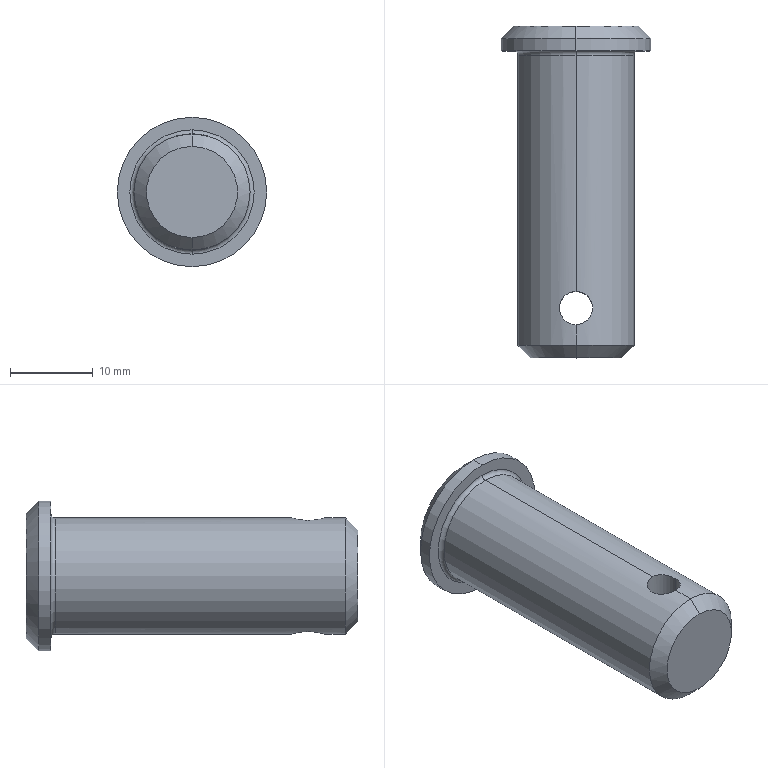Part | SolidWorks | features MirrorStock 1 | 1 solid | 15 faces | box 18 x 40 x 18 mm | volume 6181 mm3 | cylinder 6 | cone 4 | plane 3 | torus 2 | commonest cylinder face diameters 4 x2 14 x2 18 x2
STEP:
#1=CARTESIAN_POINT('',(0.,0.,-7.5));
#2=VERTEX_POINT('',#1);
#3=CARTESIAN_POINT('',(0.,0.,7.5));
#4=VERTEX_POINT('',#3);
#5=CARTESIAN_POINT('',(0.,0.,0.));
#6=DIRECTION('',(0.,-1.,0.));
#7=DIRECTION('',(0.,0.,-1.));
#8=AXIS2_PLACEMENT_3D('',#5,#6,#7);
#9=CIRCLE('',#8,7.5);
#10=EDGE_CURVE('',#2,#4,#9,.T.);
#11=ORIENTED_EDGE('',*,*,#10,.T.);
#12=CARTESIAN_POINT('',(0.,-0.5,7.));
#13=VERTEX_POINT('',#12);
#14=CARTESIAN_POINT('',(0.,-0.5,7.5));
#15=DIRECTION('',(-1.,0.,0.));
#16=DIRECTION('',(0.,0.,1.));
#17=AXIS2_PLACEMENT_3D('',#14,#15,#16);
#18=CIRCLE('',#17,0.5);
#19=EDGE_CURVE('',#4,#13,#18,.T.);
#20=ORIENTED_EDGE('',*,*,#19,.T.);
#21=CARTESIAN_POINT('',(0.,-0.5,-7.));
#22=VERTEX_POINT('',#21);
#23=CARTESIAN_POINT('',(0.,-0.5,0.));
#24=DIRECTION('',(0.,1.,0.));
#25=DIRECTION('',(0.,0.,-1.));
#26=AXIS2_PLACEMENT_3D('',#23,#24,#25);
#27=CIRCLE('',#26,7.);
#28=EDGE_CURVE('',#13,#22,#27,.T.);
#29=ORIENTED_EDGE('',*,*,#28,.T.);
#30=CARTESIAN_POINT('',(0.,-0.5,-7.5));
#31=DIRECTION('',(1.,0.,0.));
#32=DIRECTION('',(0.,0.,-1.));
#33=AXIS2_PLACEMENT_3D('',#30,#31,#32);
#34=CIRCLE('',#33,0.5);
#35=EDGE_CURVE('',#2,#22,#34,.T.);
#36=ORIENTED_EDGE('',*,*,#35,.F.);
#37=EDGE_LOOP('',(#11,#20,#29,#36));
#38=FACE_OUTER_BOUND('',#37,.T.);
#39=CARTESIAN_POINT('',(0.,-0.5,0.));
#40=DIRECTION('',(0.,1.,0.));
#41=DIRECTION('',(0.,0.,-1.));
#42=AXIS2_PLACEMENT_3D('',#39,#40,#41);
#43=TOROIDAL_SURFACE('',#42,7.5,0.5);
#44=ADVANCED_FACE('',(#38),#43,.F.);
#45=CARTESIAN_POINT('',(0.,-29.,7.));
#46=VERTEX_POINT('',#45);
#47=CARTESIAN_POINT('',(-2.,-31.,6.708));
#48=VERTEX_POINT('',#47);
#49=CARTESIAN_POINT('',(0.,-29.,7.));
#50=CARTESIAN_POINT('',(-0.1312,-29.,7.));
#51=CARTESIAN_POINT('',(-0.2645,-29.013,6.996));
#52=CARTESIAN_POINT('',(-0.5215,-29.065,6.982));
#53=CARTESIAN_POINT('',(-0.6465,-29.103,6.971));
#54=CARTESIAN_POINT('',(-1.011,-29.254,6.931));
#55=CARTESIAN_POINT('',(-1.231,-29.402,6.894));
#56=CARTESIAN_POINT('',(-1.507,-29.679,6.836));
#57=CARTESIAN_POINT('',(-1.59,-29.779,6.818));
#58=CARTESIAN_POINT('',(-1.734,-29.995,6.782));
#59=CARTESIAN_POINT('',(-1.797,-30.113,6.766));
#60=CARTESIAN_POINT('',(-1.897,-30.354,6.738));
#61=CARTESIAN_POINT('',(-1.935,-30.478,6.727));
#62=CARTESIAN_POINT('',(-1.987,-30.736,6.712));
#63=CARTESIAN_POINT('',(-2.,-30.869,6.708));
#64=CARTESIAN_POINT('',(-2.,-31.,6.708));
#65=B_SPLINE_CURVE_WITH_KNOTS('',3,(#49,#50,#51,#52,#53,#54,#55,#56,#57,#58,#59,#60,#61,#62,#63,#64),.UNSPECIFIED.,.F.,.F.,(4,2,2,2,2,2,2,4),(0.003144,0.003536,0.003929,0.004715,0.005107,0.0055,0.005893,0.006286),.UNSPECIFIED.);
#66=EDGE_CURVE('',#46,#48,#65,.T.);
#67=ORIENTED_EDGE('',*,*,#66,.T.);
#68=CARTESIAN_POINT('',(-2.,-31.,-6.708));
#69=VERTEX_POINT('',#68);
#70=CARTESIAN_POINT('',(-2.,-31.,9.));
#71=DIRECTION('',(0.,0.,-1.));
#72=VECTOR('',#71,1000.);
#73=LINE('',#70,#72);
#74=EDGE_CURVE('',#48,#69,#73,.T.);
#75=ORIENTED_EDGE('',*,*,#74,.T.);
#76=CARTESIAN_POINT('',(0.,-29.,-7.));
#77=VERTEX_POINT('',#76);
#78=CARTESIAN_POINT('',(-2.,-31.,-6.708));
#79=CARTESIAN_POINT('',(-2.,-30.869,-6.708));
#80=CARTESIAN_POINT('',(-1.987,-30.736,-6.712));
#81=CARTESIAN_POINT('',(-1.935,-30.479,-6.727));
#82=CARTESIAN_POINT('',(-1.897,-30.354,-6.738));
#83=CARTESIAN_POINT('',(-1.746,-29.989,-6.78));
#84=CARTESIAN_POINT('',(-1.598,-29.77,-6.818));
#85=CARTESIAN_POINT('',(-1.321,-29.493,-6.875));
#86=CARTESIAN_POINT('',(-1.221,-29.41,-6.894));
#87=CARTESIAN_POINT('',(-1.005,-29.266,-6.928));
#88=CARTESIAN_POINT('',(-0.8876,-29.203,-6.945));
#89=CARTESIAN_POINT('',(-0.6464,-29.103,-6.971));
#90=CARTESIAN_POINT('',(-0.5217,-29.065,-6.982));
#91=CARTESIAN_POINT('',(-0.2636,-29.013,-6.996));
#92=CARTESIAN_POINT('',(-0.1309,-29.,-7.));
#93=CARTESIAN_POINT('',(0.,-29.,-7.));
#94=B_SPLINE_CURVE_WITH_KNOTS('',3,(#78,#79,#80,#81,#82,#83,#84,#85,#86,#87,#88,#89,#90,#91,#92,#93),.UNSPECIFIED.,.F.,.F.,(4,2,2,2,2,2,2,4),(0.003144,0.003537,0.003929,0.004715,0.005108,0.0055,0.005893,0.006286),.UNSPECIFIED.);
#95=EDGE_CURVE('',#69,#77,#94,.T.);
#96=ORIENTED_EDGE('',*,*,#95,.T.);
#97=CARTESIAN_POINT('',(2.,-31.,-6.708));
#98=VERTEX_POINT('',#97);
#99=CARTESIAN_POINT('',(0.,-29.,-7.));
#100=CARTESIAN_POINT('',(0.2619,-29.,-7.));
#101=CARTESIAN_POINT('',(0.5263,-29.053,-6.984));
#102=CARTESIAN_POINT('',(0.8879,-29.203,-6.945));
#103=CARTESIAN_POINT('',(1.005,-29.266,-6.928));
#104=CARTESIAN_POINT('',(1.222,-29.411,-6.893));
#105=CARTESIAN_POINT('',(1.322,-29.493,-6.875));
#106=CARTESIAN_POINT('',(1.506,-29.678,-6.837));
#107=CARTESIAN_POINT('',(1.59,-29.78,-6.817));
#108=CARTESIAN_POINT('',(1.734,-29.995,-6.782));
#109=CARTESIAN_POINT('',(1.796,-30.11,-6.766));
#110=CARTESIAN_POINT('',(1.897,-30.354,-6.738));
#111=CARTESIAN_POINT('',(1.935,-30.479,-6.727));
#112=CARTESIAN_POINT('',(1.987,-30.735,-6.712));
#113=CARTESIAN_POINT('',(2.,-30.868,-6.708));
#114=CARTESIAN_POINT('',(2.,-31.,-6.708));
#115=B_SPLINE_CURVE_WITH_KNOTS('',3,(#99,#100,#101,#102,#103,#104,#105,#106,#107,#108,#109,#110,#111,#112,#113,#114),.UNSPECIFIED.,.F.,.F.,(4,2,2,2,2,2,2,4),(0.006286,0.007071,0.007464,0.007857,0.00825,0.008643,0.009035,0.009428),.UNSPECIFIED.);
#116=EDGE_CURVE('',#77,#98,#115,.T.);
#117=ORIENTED_EDGE('',*,*,#116,.T.);
#118=CARTESIAN_POINT('',(2.,-31.,6.708));
#119=VERTEX_POINT('',#118);
#120=CARTESIAN_POINT('',(2.,-31.,9.));
#121=DIRECTION('',(0.,0.,-1.));
#122=VECTOR('',#121,1000.);
#123=LINE('',#120,#122);
#124=EDGE_CURVE('',#119,#98,#123,.T.);
#125=ORIENTED_EDGE('',*,*,#124,.F.);
#126=CARTESIAN_POINT('',(2.,-31.,6.708));
#127=CARTESIAN_POINT('',(2.,-30.867,6.708));
#128=CARTESIAN_POINT('',(1.987,-30.737,6.712));
#129=CARTESIAN_POINT('',(1.936,-30.48,6.727));
#130=CARTESIAN_POINT('',(1.897,-30.352,6.738));
#131=CARTESIAN_POINT('',(1.796,-30.111,6.766));
#132=CARTESIAN_POINT('',(1.735,-29.996,6.782));
#133=CARTESIAN_POINT('',(1.589,-29.779,6.818));
#134=CARTESIAN_POINT('',(1.505,-29.677,6.837));
#135=CARTESIAN_POINT('',(1.23,-29.402,6.894));
#136=CARTESIAN_POINT('',(1.008,-29.253,6.931));
#137=CARTESIAN_POINT('',(0.6471,-29.103,6.971));
#138=CARTESIAN_POINT('',(0.5202,-29.064,6.982));
#139=CARTESIAN_POINT('',(0.2616,-29.013,6.996));
#140=CARTESIAN_POINT('',(0.1313,-29.,7.));
#141=CARTESIAN_POINT('',(0.,-29.,7.));
#142=B_SPLINE_CURVE_WITH_KNOTS('',3,(#126,#127,#128,#129,#130,#131,#132,#133,#134,#135,#136,#137,#138,#139,#140,#141),.UNSPECIFIED.,.F.,.F.,(4,2,2,2,2,2,2,4),(0.,0.000393,0.0007859,0.001179,0.001572,0.002358,0.002751,0.003144),.UNSPECIFIED.);
#143=EDGE_CURVE('',#119,#46,#142,.T.);
#144=ORIENTED_EDGE('',*,*,#143,.T.);
#145=EDGE_LOOP('',(#67,#75,#96,#117,#125,#144));
#146=FACE_OUTER_BOUND('',#145,.T.);
#147=CARTESIAN_POINT('',(0.,-31.,9.));
#148=DIRECTION('',(0.,0.,-1.));
#149=DIRECTION('',(1.,0.,0.));
#150=AXIS2_PLACEMENT_3D('',#147,#148,#149);
#151=CYLINDRICAL_SURFACE('',#150,2.);
#152=ADVANCED_FACE('',(#146),#151,.F.);
#153=CARTESIAN_POINT('',(0.,3.,7.5));
#154=VERTEX_POINT('',#153);
#155=CARTESIAN_POINT('',(0.,3.,-7.5));
#156=VERTEX_POINT('',#155);
#157=CARTESIAN_POINT('',(0.,3.,0.));
#158=DIRECTION('',(0.,-1.,0.));
#159=DIRECTION('',(0.,0.,-1.));
#160=AXIS2_PLACEMENT_3D('',#157,#158,#159);
#161=CIRCLE('',#160,7.5);
#162=EDGE_CURVE('',#154,#156,#161,.T.);
#163=ORIENTED_EDGE('',*,*,#162,.T.);
#164=CARTESIAN_POINT('',(0.,1.5,-9.));
#165=VERTEX_POINT('',#164);
#166=CARTESIAN_POINT('',(0.,3.,-7.5));
#167=DIRECTION('',(0.,-0.7071,-0.7071));
#168=VECTOR('',#167,1000.);
#169=LINE('',#166,#168);
#170=EDGE_CURVE('',#156,#165,#169,.T.);
#171=ORIENTED_EDGE('',*,*,#170,.T.);
#172=CARTESIAN_POINT('',(0.,1.5,9.));
#173=VERTEX_POINT('',#172);
#174=CARTESIAN_POINT('',(0.,1.5,0.));
#175=DIRECTION('',(0.,1.,0.));
#176=DIRECTION('',(0.,0.,-1.));
#177=AXIS2_PLACEMENT_3D('',#174,#175,#176);
#178=CIRCLE('',#177,9.);
#179=EDGE_CURVE('',#165,#173,#178,.T.);
#180=ORIENTED_EDGE('',*,*,#179,.T.);
#181=CARTESIAN_POINT('',(0.,3.,7.5));
#182=DIRECTION('',(0.,-0.7071,0.7071));
#183=VECTOR('',#182,1000.);
#184=LINE('',#181,#183);
#185=EDGE_CURVE('',#154,#173,#184,.T.);
#186=ORIENTED_EDGE('',*,*,#185,.F.);
#187=EDGE_LOOP('',(#163,#171,#180,#186));
#188=FACE_OUTER_BOUND('',#187,.T.);
#189=CARTESIAN_POINT('',(0.,3.,0.));
#190=DIRECTION('',(0.,-1.,0.));
#191=DIRECTION('',(0.,0.,1.));
#192=AXIS2_PLACEMENT_3D('',#189,#190,#191);
#193=CONICAL_SURFACE('',#192,7.5,0.7854);
#194=ADVANCED_FACE('',(#188),#193,.T.);
#195=CARTESIAN_POINT('',(0.,-37.,-5.5));
#196=VERTEX_POINT('',#195);
#197=CARTESIAN_POINT('',(0.,-37.,5.5));
#198=VERTEX_POINT('',#197);
#199=CARTESIAN_POINT('',(0.,-37.,0.));
#200=DIRECTION('',(0.,1.,0.));
#201=DIRECTION('',(0.,0.,1.));
#202=AXIS2_PLACEMENT_3D('',#199,#200,#201);
#203=CIRCLE('',#202,5.5);
#204=EDGE_CURVE('',#196,#198,#203,.T.);
#205=ORIENTED_EDGE('',*,*,#204,.T.);
#206=CARTESIAN_POINT('',(0.,-35.5,7.));
#207=VERTEX_POINT('',#206);
#208=CARTESIAN_POINT('',(0.,-37.,5.5));
#209=DIRECTION('',(0.,0.7071,0.7071));
#210=VECTOR('',#209,1000.);
#211=LINE('',#208,#210);
#212=EDGE_CURVE('',#198,#207,#211,.T.);
#213=ORIENTED_EDGE('',*,*,#212,.T.);
#214=CARTESIAN_POINT('',(0.,-35.5,-7.));
#215=VERTEX_POINT('',#214);
#216=CARTESIAN_POINT('',(0.,-35.5,0.));
#217=DIRECTION('',(0.,-1.,0.));
#218=DIRECTION('',(0.,0.,1.));
#219=AXIS2_PLACEMENT_3D('',#216,#217,#218);
#220=CIRCLE('',#219,7.);
#221=EDGE_CURVE('',#207,#215,#220,.T.);
#222=ORIENTED_EDGE('',*,*,#221,.T.);
#223=CARTESIAN_POINT('',(0.,-37.,-5.5));
#224=DIRECTION('',(0.,0.7071,-0.7071));
#225=VECTOR('',#224,1000.);
#226=LINE('',#223,#225);
#227=EDGE_CURVE('',#196,#215,#226,.T.);
#228=ORIENTED_EDGE('',*,*,#227,.F.);
#229=EDGE_LOOP('',(#205,#213,#222,#228));
#230=FACE_OUTER_BOUND('',#229,.T.);
#231=CARTESIAN_POINT('',(0.,-37.,0.));
#232=DIRECTION('',(0.,1.,0.));
#233=DIRECTION('',(0.,0.,-1.));
#234=AXIS2_PLACEMENT_3D('',#231,#232,#233);
#235=CONICAL_SURFACE('',#234,5.5,0.7854);
#236=ADVANCED_FACE('',(#230),#235,.T.);
#237=ORIENTED_EDGE('',*,*,#221,.F.);
#238=CARTESIAN_POINT('',(0.,-33.,7.));
#239=VERTEX_POINT('',#238);
#240=CARTESIAN_POINT('',(0.,-37.,7.));
#241=DIRECTION('',(0.,1.,0.));
#242=VECTOR('',#241,1000.);
#243=LINE('',#240,#242);
#244=EDGE_CURVE('',#207,#239,#243,.T.);
#245=ORIENTED_EDGE('',*,*,#244,.T.);
#246=CARTESIAN_POINT('',(-2.,-31.,6.708));
#247=CARTESIAN_POINT('',(-2.,-31.262,6.708));
#248=CARTESIAN_POINT('',(-1.947,-31.526,6.725));
#249=CARTESIAN_POINT('',(-1.797,-31.888,6.766));
#250=CARTESIAN_POINT('',(-1.734,-32.005,6.782));
#251=CARTESIAN_POINT('',(-1.589,-32.221,6.818));
#252=CARTESIAN_POINT('',(-1.507,-32.322,6.837));
#253=CARTESIAN_POINT('',(-1.322,-32.506,6.875));
#254=CARTESIAN_POINT('',(-1.22,-32.59,6.894));
#255=CARTESIAN_POINT('',(-1.005,-32.734,6.928));
#256=CARTESIAN_POINT('',(-0.89,-32.796,6.944));
#257=CARTESIAN_POINT('',(-0.646,-32.897,6.971));
#258=CARTESIAN_POINT('',(-0.5208,-32.935,6.982));
#259=CARTESIAN_POINT('',(-0.2645,-32.987,6.996));
#260=CARTESIAN_POINT('',(-0.1318,-33.,7.));
#261=CARTESIAN_POINT('',(0.,-33.,7.));
#262=B_SPLINE_CURVE_WITH_KNOTS('',3,(#246,#247,#248,#249,#250,#251,#252,#253,#254,#255,#256,#257,#258,#259,#260,#261),.UNSPECIFIED.,.F.,.F.,(4,2,2,2,2,2,2,4),(0.006286,0.007071,0.007464,0.007857,0.00825,0.008642,0.009035,0.009428),.UNSPECIFIED.);
#263=EDGE_CURVE('',#48,#239,#262,.T.);
#264=ORIENTED_EDGE('',*,*,#263,.F.);
#265=ORIENTED_EDGE('',*,*,#66,.F.);
#266=CARTESIAN_POINT('',(0.,-37.,7.));
#267=DIRECTION('',(0.,1.,0.));
#268=VECTOR('',#267,1000.);
#269=LINE('',#266,#268);
#270=EDGE_CURVE('',#46,#13,#269,.T.);
#271=ORIENTED_EDGE('',*,*,#270,.T.);
#272=CARTESIAN_POINT('',(0.,-0.5,0.));
#273=DIRECTION('',(0.,1.,0.));
#274=DIRECTION('',(0.,0.,-1.));
#275=AXIS2_PLACEMENT_3D('',#272,#273,#274);
#276=CIRCLE('',#275,7.);
#277=EDGE_CURVE('',#22,#13,#276,.T.);
#278=ORIENTED_EDGE('',*,*,#277,.F.);
#279=CARTESIAN_POINT('',(0.,-37.,-7.));
#280=DIRECTION('',(0.,1.,0.));
#281=VECTOR('',#280,1000.);
#282=LINE('',#279,#281);
#283=EDGE_CURVE('',#77,#22,#282,.T.);
#284=ORIENTED_EDGE('',*,*,#283,.F.);
#285=ORIENTED_EDGE('',*,*,#95,.F.);
#286=CARTESIAN_POINT('',(0.,-33.,-7.));
#287=VERTEX_POINT('',#286);
#288=CARTESIAN_POINT('',(0.,-33.,-7.));
#289=CARTESIAN_POINT('',(-0.1329,-33.,-7.));
#290=CARTESIAN_POINT('',(-0.2635,-32.987,-6.996));
#291=CARTESIAN_POINT('',(-0.5202,-32.936,-6.982));
#292=CARTESIAN_POINT('',(-0.6476,-32.897,-6.971));
#293=CARTESIAN_POINT('',(-0.8896,-32.796,-6.944));
#294=CARTESIAN_POINT('',(-1.004,-32.735,-6.928));
#295=CARTESIAN_POINT('',(-1.221,-32.589,-6.894));
#296=CARTESIAN_POINT('',(-1.323,-32.505,-6.874));
#297=CARTESIAN_POINT('',(-1.598,-32.23,-6.818));
#298=CARTESIAN_POINT('',(-1.747,-32.008,-6.779));
#299=CARTESIAN_POINT('',(-1.897,-31.647,-6.738));
#300=CARTESIAN_POINT('',(-1.936,-31.52,-6.727));
#301=CARTESIAN_POINT('',(-1.987,-31.262,-6.712));
#302=CARTESIAN_POINT('',(-2.,-31.131,-6.708));
#303=CARTESIAN_POINT('',(-2.,-31.,-6.708));
#304=B_SPLINE_CURVE_WITH_KNOTS('',3,(#288,#289,#290,#291,#292,#293,#294,#295,#296,#297,#298,#299,#300,#301,#302,#303),.UNSPECIFIED.,.F.,.F.,(4,2,2,2,2,2,2,4),(0.,0.000393,0.000786,0.001179,0.001572,0.002358,0.002751,0.003144),.UNSPECIFIED.);
#305=EDGE_CURVE('',#287,#69,#304,.T.);
#306=ORIENTED_EDGE('',*,*,#305,.F.);
#307=CARTESIAN_POINT('',(0.,-37.,-7.));
#308=DIRECTION('',(0.,1.,0.));
#309=VECTOR('',#308,1000.);
#310=LINE('',#307,#309);
#311=EDGE_CURVE('',#215,#287,#310,.T.);
#312=ORIENTED_EDGE('',*,*,#311,.F.);
#313=EDGE_LOOP('',(#237,#245,#264,#265,#271,#278,#284,#285,#306,#312));
#314=FACE_OUTER_BOUND('',#313,.T.);
#315=CARTESIAN_POINT('',(0.,-37.,0.));
#316=DIRECTION('',(0.,1.,0.));
#317=DIRECTION('',(0.,0.,-1.));
#318=AXIS2_PLACEMENT_3D('',#315,#316,#317);
#319=CYLINDRICAL_SURFACE('',#318,7.);
#320=ADVANCED_FACE('',(#314),#319,.T.);
#321=ORIENTED_EDGE('',*,*,#179,.F.);
#322=CARTESIAN_POINT('',(0.,0.,-9.));
#323=VERTEX_POINT('',#322);
#324=CARTESIAN_POINT('',(0.,3.,-9.));
#325=DIRECTION('',(0.,-1.,0.));
#326=VECTOR('',#325,1000.);
#327=LINE('',#324,#326);
#328=EDGE_CURVE('',#165,#323,#327,.T.);
#329=ORIENTED_EDGE('',*,*,#328,.T.);
#330=CARTESIAN_POINT('',(0.,0.,9.));
#331=VERTEX_POINT('',#330);
#332=CARTESIAN_POINT('',(0.,0.,0.));
#333=DIRECTION('',(0.,-1.,0.));
#334=DIRECTION('',(0.,0.,-1.));
#335=AXIS2_PLACEMENT_3D('',#332,#333,#334);
#336=CIRCLE('',#335,9.);
#337=EDGE_CURVE('',#331,#323,#336,.T.);
#338=ORIENTED_EDGE('',*,*,#337,.F.);
#339=CARTESIAN_POINT('',(0.,3.,9.));
#340=DIRECTION('',(0.,-1.,0.));
#341=VECTOR('',#340,1000.);
#342=LINE('',#339,#341);
#343=EDGE_CURVE('',#173,#331,#342,.T.);
#344=ORIENTED_EDGE('',*,*,#343,.F.);
#345=EDGE_LOOP('',(#321,#329,#338,#344));
#346=FACE_OUTER_BOUND('',#345,.T.);
#347=CARTESIAN_POINT('',(0.,3.,0.));
#348=DIRECTION('',(0.,-1.,0.));
#349=DIRECTION('',(0.,0.,1.));
#350=AXIS2_PLACEMENT_3D('',#347,#348,#349);
#351=CYLINDRICAL_SURFACE('',#350,9.);
#352=ADVANCED_FACE('',(#346),#351,.T.);
#353=ORIENTED_EDGE('',*,*,#328,.F.);
#354=CARTESIAN_POINT('',(0.,1.5,0.));
#355=DIRECTION('',(0.,1.,0.));
#356=DIRECTION('',(0.,0.,-1.));
#357=AXIS2_PLACEMENT_3D('',#354,#355,#356);
#358=CIRCLE('',#357,9.);
#359=EDGE_CURVE('',#173,#165,#358,.T.);
#360=ORIENTED_EDGE('',*,*,#359,.F.);
#361=ORIENTED_EDGE('',*,*,#343,.T.);
#362=CARTESIAN_POINT('',(0.,0.,0.));
#363=DIRECTION('',(0.,-1.,0.));
#364=DIRECTION('',(0.,0.,-1.));
#365=AXIS2_PLACEMENT_3D('',#362,#363,#364);
#366=CIRCLE('',#365,9.);
#367=EDGE_CURVE('',#323,#331,#366,.T.);
#368=ORIENTED_EDGE('',*,*,#367,.F.);
#369=EDGE_LOOP('',(#353,#360,#361,#368));
#370=FACE_OUTER_BOUND('',#369,.T.);
#371=CARTESIAN_POINT('',(0.,3.,0.));
#372=DIRECTION('',(0.,-1.,0.));
#373=DIRECTION('',(0.,0.,1.));
#374=AXIS2_PLACEMENT_3D('',#371,#372,#373);
#375=CYLINDRICAL_SURFACE('',#374,9.);
#376=ADVANCED_FACE('',(#370),#375,.T.);
#377=ORIENTED_EDGE('',*,*,#162,.F.);
#378=CARTESIAN_POINT('',(0.,3.,0.));
#379=DIRECTION('',(0.,-1.,0.));
#380=DIRECTION('',(0.,0.,-1.));
#381=AXIS2_PLACEMENT_3D('',#378,#379,#380);
#382=CIRCLE('',#381,7.5);
#383=EDGE_CURVE('',#156,#154,#382,.T.);
#384=ORIENTED_EDGE('',*,*,#383,.F.);
#385=EDGE_LOOP('',(#377,#384));
#386=FACE_OUTER_BOUND('',#385,.T.);
#387=CARTESIAN_POINT('',(0.,3.,0.));
#388=DIRECTION('',(0.,1.,0.));
#389=DIRECTION('',(0.,0.,-1.));
#390=AXIS2_PLACEMENT_3D('',#387,#388,#389);
#391=PLANE('',#390);
#392=ADVANCED_FACE('',(#386),#391,.T.);
#393=ORIENTED_EDGE('',*,*,#10,.F.);
#394=CARTESIAN_POINT('',(0.,0.,0.));
#395=DIRECTION('',(0.,-1.,0.));
#396=DIRECTION('',(0.,0.,-1.));
#397=AXIS2_PLACEMENT_3D('',#394,#395,#396);
#398=CIRCLE('',#397,7.5);
#399=EDGE_CURVE('',#4,#2,#398,.T.);
#400=ORIENTED_EDGE('',*,*,#399,.F.);
#401=EDGE_LOOP('',(#393,#400));
#402=FACE_BOUND('',#401,.T.);
#403=ORIENTED_EDGE('',*,*,#337,.T.);
#404=ORIENTED_EDGE('',*,*,#367,.T.);
#405=EDGE_LOOP('',(#403,#404));
#406=FACE_OUTER_BOUND('',#405,.T.);
#407=CARTESIAN_POINT('',(0.,0.,0.));
#408=DIRECTION('',(0.,1.,0.));
#409=DIRECTION('',(0.,0.,-1.));
#410=AXIS2_PLACEMENT_3D('',#407,#408,#409);
#411=PLANE('',#410);
#412=ADVANCED_FACE('',(#402,#406),#411,.F.);
#413=ORIENTED_EDGE('',*,*,#244,.F.);
#414=CARTESIAN_POINT('',(0.,-35.5,0.));
#415=DIRECTION('',(0.,-1.,0.));
#416=DIRECTION('',(0.,0.,1.));
#417=AXIS2_PLACEMENT_3D('',#414,#415,#416);
#418=CIRCLE('',#417,7.);
#419=EDGE_CURVE('',#215,#207,#418,.T.);
#420=ORIENTED_EDGE('',*,*,#419,.F.);
#421=ORIENTED_EDGE('',*,*,#311,.T.);
#422=CARTESIAN_POINT('',(2.,-31.,-6.708));
#423=CARTESIAN_POINT('',(2.,-31.132,-6.708));
#424=CARTESIAN_POINT('',(1.987,-31.262,-6.712));
#425=CARTESIAN_POINT('',(1.936,-31.519,-6.727));
#426=CARTESIAN_POINT('',(1.897,-31.647,-6.738));
#427=CARTESIAN_POINT('',(1.747,-32.008,-6.779));
#428=CARTESIAN_POINT('',(1.598,-32.23,-6.818));
#429=CARTESIAN_POINT('',(1.323,-32.505,-6.874));
#430=CARTESIAN_POINT('',(1.221,-32.589,-6.894));
#431=CARTESIAN_POINT('',(1.004,-32.735,-6.928));
#432=CARTESIAN_POINT('',(0.8896,-32.796,-6.944));
#433=CARTESIAN_POINT('',(0.6486,-32.896,-6.971));
#434=CARTESIAN_POINT('',(0.521,-32.935,-6.982));
#435=CARTESIAN_POINT('',(0.2636,-32.987,-6.996));
#436=CARTESIAN_POINT('',(0.1328,-33.,-7.));
#437=CARTESIAN_POINT('',(0.,-33.,-7.));
#438=B_SPLINE_CURVE_WITH_KNOTS('',3,(#422,#423,#424,#425,#426,#427,#428,#429,#430,#431,#432,#433,#434,#435,#436,#437),.UNSPECIFIED.,.F.,.F.,(4,2,2,2,2,2,2,4),(0.009428,0.009821,0.01021,0.011,0.01139,0.01178,0.01218,0.01257),.UNSPECIFIED.);
#439=EDGE_CURVE('',#98,#287,#438,.T.);
#440=ORIENTED_EDGE('',*,*,#439,.F.);
#441=ORIENTED_EDGE('',*,*,#116,.F.);
#442=ORIENTED_EDGE('',*,*,#283,.T.);
#443=ORIENTED_EDGE('',*,*,#28,.F.);
#444=ORIENTED_EDGE('',*,*,#270,.F.);
#445=ORIENTED_EDGE('',*,*,#143,.F.);
#446=CARTESIAN_POINT('',(0.,-33.,7.));
#447=CARTESIAN_POINT('',(0.1318,-33.,7.));
#448=CARTESIAN_POINT('',(0.2621,-32.987,6.996));
#449=CARTESIAN_POINT('',(0.5195,-32.936,6.982));
#450=CARTESIAN_POINT('',(0.6471,-32.897,6.971));
#451=CARTESIAN_POINT('',(1.009,-32.747,6.931));
#452=CARTESIAN_POINT('',(1.23,-32.598,6.894));
#453=CARTESIAN_POINT('',(1.506,-32.323,6.837));
#454=CARTESIAN_POINT('',(1.589,-32.221,6.818));
#455=CARTESIAN_POINT('',(1.735,-32.004,6.782));
#456=CARTESIAN_POINT('',(1.796,-31.89,6.766));
#457=CARTESIAN_POINT('',(1.896,-31.649,6.738));
#458=CARTESIAN_POINT('',(1.935,-31.521,6.727));
#459=CARTESIAN_POINT('',(1.987,-31.264,6.712));
#460=CARTESIAN_POINT('',(2.,-31.133,6.708));
#461=CARTESIAN_POINT('',(2.,-31.,6.708));
#462=B_SPLINE_CURVE_WITH_KNOTS('',3,(#446,#447,#448,#449,#450,#451,#452,#453,#454,#455,#456,#457,#458,#459,#460,#461),.UNSPECIFIED.,.F.,.F.,(4,2,2,2,2,2,2,4),(0.009428,0.009821,0.01021,0.011,0.01139,0.01178,0.01218,0.01257),.UNSPECIFIED.);
#463=EDGE_CURVE('',#239,#119,#462,.T.);
#464=ORIENTED_EDGE('',*,*,#463,.F.);
#465=EDGE_LOOP('',(#413,#420,#421,#440,#441,#442,#443,#444,#445,#464));
#466=FACE_OUTER_BOUND('',#465,.T.);
#467=CARTESIAN_POINT('',(0.,-37.,0.));
#468=DIRECTION('',(0.,1.,0.));
#469=DIRECTION('',(0.,0.,-1.));
#470=AXIS2_PLACEMENT_3D('',#467,#468,#469);
#471=CYLINDRICAL_SURFACE('',#470,7.);
#472=ADVANCED_FACE('',(#466),#471,.T.);
#473=ORIENTED_EDGE('',*,*,#204,.F.);
#474=CARTESIAN_POINT('',(0.,-37.,0.));
#475=DIRECTION('',(0.,1.,0.));
#476=DIRECTION('',(0.,0.,1.));
#477=AXIS2_PLACEMENT_3D('',#474,#475,#476);
#478=CIRCLE('',#477,5.5);
#479=EDGE_CURVE('',#198,#196,#478,.T.);
#480=ORIENTED_EDGE('',*,*,#479,.F.);
#481=EDGE_LOOP('',(#473,#480));
#482=FACE_OUTER_BOUND('',#481,.T.);
#483=CARTESIAN_POINT('',(0.,-37.,0.));
#484=DIRECTION('',(0.,-1.,0.));
#485=DIRECTION('',(0.,0.,1.));
#486=AXIS2_PLACEMENT_3D('',#483,#484,#485);
#487=PLANE('',#486);
#488=ADVANCED_FACE('',(#482),#487,.T.);
#489=ORIENTED_EDGE('',*,*,#212,.F.);
#490=ORIENTED_EDGE('',*,*,#479,.T.);
#491=ORIENTED_EDGE('',*,*,#227,.T.);
#492=ORIENTED_EDGE('',*,*,#419,.T.);
#493=EDGE_LOOP('',(#489,#490,#491,#492));
#494=FACE_OUTER_BOUND('',#493,.T.);
#495=CARTESIAN_POINT('',(0.,-37.,0.));
#496=DIRECTION('',(0.,1.,0.));
#497=DIRECTION('',(0.,0.,-1.));
#498=AXIS2_PLACEMENT_3D('',#495,#496,#497);
#499=CONICAL_SURFACE('',#498,5.5,0.7854);
#500=ADVANCED_FACE('',(#494),#499,.T.);
#501=ORIENTED_EDGE('',*,*,#170,.F.);
#502=ORIENTED_EDGE('',*,*,#383,.T.);
#503=ORIENTED_EDGE('',*,*,#185,.T.);
#504=ORIENTED_EDGE('',*,*,#359,.T.);
#505=EDGE_LOOP('',(#501,#502,#503,#504));
#506=FACE_OUTER_BOUND('',#505,.T.);
#507=CARTESIAN_POINT('',(0.,3.,0.));
#508=DIRECTION('',(0.,-1.,0.));
#509=DIRECTION('',(0.,0.,1.));
#510=AXIS2_PLACEMENT_3D('',#507,#508,#509);
#511=CONICAL_SURFACE('',#510,7.5,0.7854);
#512=ADVANCED_FACE('',(#506),#511,.T.);
#513=ORIENTED_EDGE('',*,*,#74,.F.);
#514=ORIENTED_EDGE('',*,*,#263,.T.);
#515=ORIENTED_EDGE('',*,*,#463,.T.);
#516=ORIENTED_EDGE('',*,*,#124,.T.);
#517=ORIENTED_EDGE('',*,*,#439,.T.);
#518=ORIENTED_EDGE('',*,*,#305,.T.);
#519=EDGE_LOOP('',(#513,#514,#515,#516,#517,#518));
#520=FACE_OUTER_BOUND('',#519,.T.);
#521=CARTESIAN_POINT('',(0.,-31.,9.));
#522=DIRECTION('',(0.,0.,-1.));
#523=DIRECTION('',(1.,0.,0.));
#524=AXIS2_PLACEMENT_3D('',#521,#522,#523);
#525=CYLINDRICAL_SURFACE('',#524,2.);
#526=ADVANCED_FACE('',(#520),#525,.F.);
#527=ORIENTED_EDGE('',*,*,#19,.F.);
#528=ORIENTED_EDGE('',*,*,#399,.T.);
#529=ORIENTED_EDGE('',*,*,#35,.T.);
#530=ORIENTED_EDGE('',*,*,#277,.T.);
#531=EDGE_LOOP('',(#527,#528,#529,#530));
#532=FACE_OUTER_BOUND('',#531,.T.);
#533=CARTESIAN_POINT('',(0.,-0.5,0.));
#534=DIRECTION('',(0.,1.,0.));
#535=DIRECTION('',(0.,0.,-1.));
#536=AXIS2_PLACEMENT_3D('',#533,#534,#535);
#537=TOROIDAL_SURFACE('',#536,7.5,0.5);
#538=ADVANCED_FACE('',(#532),#537,.F.);
#539=CLOSED_SHELL('',(#44,#152,#194,#236,#320,#352,#376,#392,#412,#472,#488,#500,#512,#526,#538));
#540=MANIFOLD_SOLID_BREP('',#539);
#541=CARTESIAN_POINT('',(0.,0.,0.));
#542=DIRECTION('',(0.,0.,1.));
#543=DIRECTION('',(1.,0.,0.));
#544=AXIS2_PLACEMENT_3D('',#541,#542,#543);
#545=(LENGTH_UNIT()NAMED_UNIT(*)SI_UNIT(.MILLI.,.METRE.));
#546=UNCERTAINTY_MEASURE_WITH_UNIT(LENGTH_MEASURE(0.00001),#545,'','');
#547=(NAMED_UNIT(*)PLANE_ANGLE_UNIT()SI_UNIT($,.RADIAN.));
#548=(NAMED_UNIT(*)SI_UNIT($,.STERADIAN.)SOLID_ANGLE_UNIT());
#549=(GEOMETRIC_REPRESENTATION_CONTEXT(3)GLOBAL_UNCERTAINTY_ASSIGNED_CONTEXT((#546))GLOBAL_UNIT_ASSIGNED_CONTEXT((#545,#547,#548))REPRESENTATION_CONTEXT('',''));
#550=ADVANCED_BREP_SHAPE_REPRESENTATION('',(#540,#544),#549);